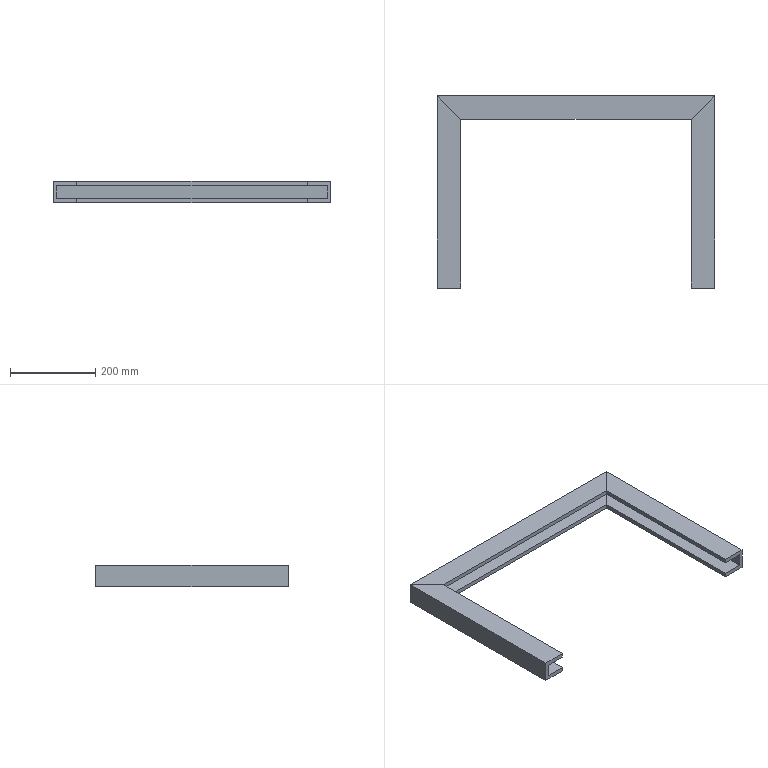Part | STEP file | kunza | 1 solid | 26 faces | box 650 x 450 x 50 mm | volume 1951319 mm3 | plane 26